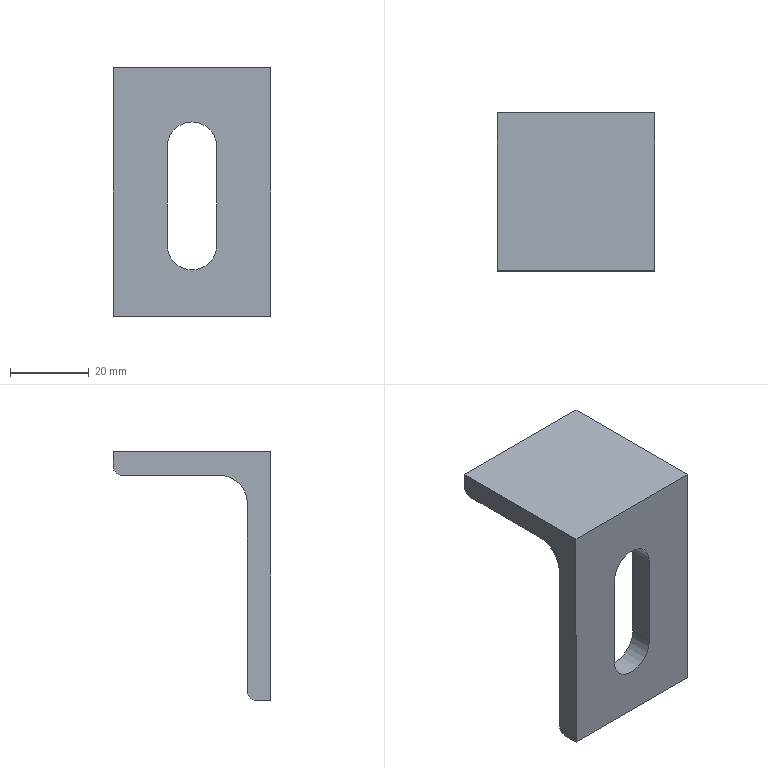Part | SolidWorks | features 3DProfileFeature 1, Cut 1, WeldMemberFeat 1, WeldmentFeature 1 | 1 solid | 16 faces | box 40 x 40 x 63 mm | volume 20996 mm3 | plane 10 | cylinder 6 | commonest cylinder face diameters 12.5 x3 4.667 x2 14 x1
STEP:
#1=CARTESIAN_POINT('',(200.,114.,-13.75));
#2=VERTEX_POINT('',#1);
#3=CARTESIAN_POINT('',(206.25,114.,-20.));
#4=VERTEX_POINT('',#3);
#5=CARTESIAN_POINT('',(200.,114.,-20.));
#6=DIRECTION('',(0.,1.,0.));
#7=DIRECTION('',(0.,0.,1.));
#8=AXIS2_PLACEMENT_3D('',#5,#6,#7);
#9=CIRCLE('',#8,6.25);
#10=EDGE_CURVE('',#2,#4,#9,.T.);
#11=ORIENTED_EDGE('',*,*,#10,.F.);
#12=CARTESIAN_POINT('',(200.,120.,-13.75));
#13=VERTEX_POINT('',#12);
#14=CARTESIAN_POINT('',(200.,110.,-13.75));
#15=DIRECTION('',(0.,1.,0.));
#16=VECTOR('',#15,1000.);
#17=LINE('',#14,#16);
#18=EDGE_CURVE('',#2,#13,#17,.T.);
#19=ORIENTED_EDGE('',*,*,#18,.T.);
#20=CARTESIAN_POINT('',(206.25,120.,-20.));
#21=VERTEX_POINT('',#20);
#22=CARTESIAN_POINT('',(200.,120.,-20.));
#23=DIRECTION('',(0.,1.,0.));
#24=DIRECTION('',(0.,0.,1.));
#25=AXIS2_PLACEMENT_3D('',#22,#23,#24);
#26=CIRCLE('',#25,6.25);
#27=EDGE_CURVE('',#13,#21,#26,.T.);
#28=ORIENTED_EDGE('',*,*,#27,.T.);
#29=CARTESIAN_POINT('',(206.25,110.,-20.));
#30=DIRECTION('',(0.,1.,0.));
#31=VECTOR('',#30,1000.);
#32=LINE('',#29,#31);
#33=EDGE_CURVE('',#4,#21,#32,.T.);
#34=ORIENTED_EDGE('',*,*,#33,.F.);
#35=EDGE_LOOP('',(#11,#19,#28,#34));
#36=FACE_OUTER_BOUND('',#35,.T.);
#37=CARTESIAN_POINT('',(200.,110.,-20.));
#38=DIRECTION('',(0.,1.,0.));
#39=DIRECTION('',(0.,0.,1.));
#40=AXIS2_PLACEMENT_3D('',#37,#38,#39);
#41=CYLINDRICAL_SURFACE('',#40,6.25);
#42=ADVANCED_FACE('',(#36),#41,.F.);
#43=CARTESIAN_POINT('',(220.,114.,0.));
#44=VERTEX_POINT('',#43);
#45=CARTESIAN_POINT('',(220.,154.,0.));
#46=VERTEX_POINT('',#45);
#47=CARTESIAN_POINT('',(220.,154.,0.));
#48=DIRECTION('',(0.,1.,0.));
#49=VECTOR('',#48,1000.);
#50=LINE('',#47,#49);
#51=EDGE_CURVE('',#44,#46,#50,.T.);
#52=ORIENTED_EDGE('',*,*,#51,.T.);
#53=CARTESIAN_POINT('',(180.,154.,0.));
#54=VERTEX_POINT('',#53);
#55=CARTESIAN_POINT('',(180.,154.,0.));
#56=DIRECTION('',(1.,0.,0.));
#57=VECTOR('',#56,1000.);
#58=LINE('',#55,#57);
#59=EDGE_CURVE('',#54,#46,#58,.T.);
#60=ORIENTED_EDGE('',*,*,#59,.F.);
#61=CARTESIAN_POINT('',(180.,114.,0.));
#62=VERTEX_POINT('',#61);
#63=CARTESIAN_POINT('',(180.,154.,0.));
#64=DIRECTION('',(0.,1.,0.));
#65=VECTOR('',#64,1000.);
#66=LINE('',#63,#65);
#67=EDGE_CURVE('',#62,#54,#66,.T.);
#68=ORIENTED_EDGE('',*,*,#67,.F.);
#69=CARTESIAN_POINT('',(180.,114.,0.));
#70=DIRECTION('',(1.,0.,0.));
#71=VECTOR('',#70,1000.);
#72=LINE('',#69,#71);
#73=EDGE_CURVE('',#62,#44,#72,.T.);
#74=ORIENTED_EDGE('',*,*,#73,.T.);
#75=EDGE_LOOP('',(#52,#60,#68,#74));
#76=FACE_OUTER_BOUND('',#75,.T.);
#77=CARTESIAN_POINT('',(180.,154.,0.));
#78=DIRECTION('',(0.,0.,-1.));
#79=DIRECTION('',(0.,1.,0.));
#80=AXIS2_PLACEMENT_3D('',#77,#78,#79);
#81=PLANE('',#80);
#82=ADVANCED_FACE('',(#76),#81,.F.);
#83=CARTESIAN_POINT('',(220.,154.,-3.667));
#84=VERTEX_POINT('',#83);
#85=CARTESIAN_POINT('',(220.,154.,0.));
#86=DIRECTION('',(0.,0.,-1.));
#87=VECTOR('',#86,1000.);
#88=LINE('',#85,#87);
#89=EDGE_CURVE('',#46,#84,#88,.T.);
#90=ORIENTED_EDGE('',*,*,#89,.T.);
#91=CARTESIAN_POINT('',(180.,154.,-3.667));
#92=VERTEX_POINT('',#91);
#93=CARTESIAN_POINT('',(180.,154.,-3.667));
#94=DIRECTION('',(1.,0.,0.));
#95=VECTOR('',#94,1000.);
#96=LINE('',#93,#95);
#97=EDGE_CURVE('',#92,#84,#96,.T.);
#98=ORIENTED_EDGE('',*,*,#97,.F.);
#99=CARTESIAN_POINT('',(180.,154.,0.));
#100=DIRECTION('',(0.,0.,-1.));
#101=VECTOR('',#100,1000.);
#102=LINE('',#99,#101);
#103=EDGE_CURVE('',#54,#92,#102,.T.);
#104=ORIENTED_EDGE('',*,*,#103,.F.);
#105=ORIENTED_EDGE('',*,*,#59,.T.);
#106=EDGE_LOOP('',(#90,#98,#104,#105));
#107=FACE_OUTER_BOUND('',#106,.T.);
#108=CARTESIAN_POINT('',(180.,154.,0.));
#109=DIRECTION('',(0.,-1.,0.));
#110=DIRECTION('',(0.,0.,-1.));
#111=AXIS2_PLACEMENT_3D('',#108,#109,#110);
#112=PLANE('',#111);
#113=ADVANCED_FACE('',(#107),#112,.F.);
#114=CARTESIAN_POINT('',(220.,151.667,-6.));
#115=VERTEX_POINT('',#114);
#116=CARTESIAN_POINT('',(220.,151.667,-3.667));
#117=DIRECTION('',(-1.,0.,0.));
#118=DIRECTION('',(0.,0.,1.));
#119=AXIS2_PLACEMENT_3D('',#116,#117,#118);
#120=CIRCLE('',#119,2.333);
#121=EDGE_CURVE('',#84,#115,#120,.T.);
#122=ORIENTED_EDGE('',*,*,#121,.T.);
#123=CARTESIAN_POINT('',(180.,151.667,-6.));
#124=VERTEX_POINT('',#123);
#125=CARTESIAN_POINT('',(180.,151.667,-6.));
#126=DIRECTION('',(1.,0.,0.));
#127=VECTOR('',#126,1000.);
#128=LINE('',#125,#127);
#129=EDGE_CURVE('',#124,#115,#128,.T.);
#130=ORIENTED_EDGE('',*,*,#129,.F.);
#131=CARTESIAN_POINT('',(180.,151.667,-3.667));
#132=DIRECTION('',(-1.,0.,0.));
#133=DIRECTION('',(0.,0.,1.));
#134=AXIS2_PLACEMENT_3D('',#131,#132,#133);
#135=CIRCLE('',#134,2.333);
#136=EDGE_CURVE('',#92,#124,#135,.T.);
#137=ORIENTED_EDGE('',*,*,#136,.F.);
#138=ORIENTED_EDGE('',*,*,#97,.T.);
#139=EDGE_LOOP('',(#122,#130,#137,#138));
#140=FACE_OUTER_BOUND('',#139,.T.);
#141=CARTESIAN_POINT('',(180.,151.667,-3.667));
#142=DIRECTION('',(1.,0.,0.));
#143=DIRECTION('',(0.,0.,-1.));
#144=AXIS2_PLACEMENT_3D('',#141,#142,#143);
#145=CYLINDRICAL_SURFACE('',#144,2.333);
#146=ADVANCED_FACE('',(#140),#145,.T.);
#147=CARTESIAN_POINT('',(220.,127.,-6.));
#148=VERTEX_POINT('',#147);
#149=CARTESIAN_POINT('',(220.,127.,-6.));
#150=DIRECTION('',(0.,-1.,0.));
#151=VECTOR('',#150,1000.);
#152=LINE('',#149,#151);
#153=EDGE_CURVE('',#115,#148,#152,.T.);
#154=ORIENTED_EDGE('',*,*,#153,.T.);
#155=CARTESIAN_POINT('',(180.,127.,-6.));
#156=VERTEX_POINT('',#155);
#157=CARTESIAN_POINT('',(180.,127.,-6.));
#158=DIRECTION('',(1.,0.,0.));
#159=VECTOR('',#158,1000.);
#160=LINE('',#157,#159);
#161=EDGE_CURVE('',#156,#148,#160,.T.);
#162=ORIENTED_EDGE('',*,*,#161,.F.);
#163=CARTESIAN_POINT('',(180.,127.,-6.));
#164=DIRECTION('',(0.,-1.,0.));
#165=VECTOR('',#164,1000.);
#166=LINE('',#163,#165);
#167=EDGE_CURVE('',#124,#156,#166,.T.);
#168=ORIENTED_EDGE('',*,*,#167,.F.);
#169=ORIENTED_EDGE('',*,*,#129,.T.);
#170=EDGE_LOOP('',(#154,#162,#168,#169));
#171=FACE_OUTER_BOUND('',#170,.T.);
#172=CARTESIAN_POINT('',(180.,127.,-6.));
#173=DIRECTION('',(0.,0.,1.));
#174=DIRECTION('',(0.,-1.,0.));
#175=AXIS2_PLACEMENT_3D('',#172,#173,#174);
#176=PLANE('',#175);
#177=ADVANCED_FACE('',(#171),#176,.F.);
#178=CARTESIAN_POINT('',(220.,120.,-13.));
#179=VERTEX_POINT('',#178);
#180=CARTESIAN_POINT('',(220.,127.,-13.));
#181=DIRECTION('',(1.,0.,0.));
#182=DIRECTION('',(0.,0.,-1.));
#183=AXIS2_PLACEMENT_3D('',#180,#181,#182);
#184=CIRCLE('',#183,7.);
#185=EDGE_CURVE('',#148,#179,#184,.T.);
#186=ORIENTED_EDGE('',*,*,#185,.T.);
#187=CARTESIAN_POINT('',(180.,120.,-13.));
#188=VERTEX_POINT('',#187);
#189=CARTESIAN_POINT('',(180.,120.,-13.));
#190=DIRECTION('',(1.,0.,0.));
#191=VECTOR('',#190,1000.);
#192=LINE('',#189,#191);
#193=EDGE_CURVE('',#188,#179,#192,.T.);
#194=ORIENTED_EDGE('',*,*,#193,.F.);
#195=CARTESIAN_POINT('',(180.,127.,-13.));
#196=DIRECTION('',(1.,0.,0.));
#197=DIRECTION('',(0.,0.,-1.));
#198=AXIS2_PLACEMENT_3D('',#195,#196,#197);
#199=CIRCLE('',#198,7.);
#200=EDGE_CURVE('',#156,#188,#199,.T.);
#201=ORIENTED_EDGE('',*,*,#200,.F.);
#202=ORIENTED_EDGE('',*,*,#161,.T.);
#203=EDGE_LOOP('',(#186,#194,#201,#202));
#204=FACE_OUTER_BOUND('',#203,.T.);
#205=CARTESIAN_POINT('',(180.,127.,-13.));
#206=DIRECTION('',(1.,0.,0.));
#207=DIRECTION('',(0.,0.,-1.));
#208=AXIS2_PLACEMENT_3D('',#205,#206,#207);
#209=CYLINDRICAL_SURFACE('',#208,7.);
#210=ADVANCED_FACE('',(#204),#209,.F.);
#211=CARTESIAN_POINT('',(193.75,120.,-45.));
#212=VERTEX_POINT('',#211);
#213=CARTESIAN_POINT('',(193.75,120.,-20.));
#214=VERTEX_POINT('',#213);
#215=CARTESIAN_POINT('',(193.75,120.,-45.));
#216=DIRECTION('',(0.,0.,1.));
#217=VECTOR('',#216,1000.);
#218=LINE('',#215,#217);
#219=EDGE_CURVE('',#212,#214,#218,.T.);
#220=ORIENTED_EDGE('',*,*,#219,.F.);
#221=CARTESIAN_POINT('',(206.25,120.,-45.));
#222=VERTEX_POINT('',#221);
#223=CARTESIAN_POINT('',(200.,120.,-45.));
#224=DIRECTION('',(0.,1.,0.));
#225=DIRECTION('',(0.,0.,1.));
#226=AXIS2_PLACEMENT_3D('',#223,#224,#225);
#227=CIRCLE('',#226,6.25);
#228=EDGE_CURVE('',#222,#212,#227,.T.);
#229=ORIENTED_EDGE('',*,*,#228,.F.);
#230=CARTESIAN_POINT('',(206.25,120.,-45.));
#231=DIRECTION('',(0.,0.,-1.));
#232=VECTOR('',#231,1000.);
#233=LINE('',#230,#232);
#234=EDGE_CURVE('',#21,#222,#233,.T.);
#235=ORIENTED_EDGE('',*,*,#234,.F.);
#236=ORIENTED_EDGE('',*,*,#27,.F.);
#237=CARTESIAN_POINT('',(200.,120.,-20.));
#238=DIRECTION('',(0.,1.,0.));
#239=DIRECTION('',(0.,0.,1.));
#240=AXIS2_PLACEMENT_3D('',#237,#238,#239);
#241=CIRCLE('',#240,6.25);
#242=EDGE_CURVE('',#214,#13,#241,.T.);
#243=ORIENTED_EDGE('',*,*,#242,.F.);
#244=EDGE_LOOP('',(#220,#229,#235,#236,#243));
#245=FACE_BOUND('',#244,.T.);
#246=CARTESIAN_POINT('',(220.,120.,-60.667));
#247=VERTEX_POINT('',#246);
#248=CARTESIAN_POINT('',(220.,120.,-60.667));
#249=DIRECTION('',(0.,0.,-1.));
#250=VECTOR('',#249,1000.);
#251=LINE('',#248,#250);
#252=EDGE_CURVE('',#179,#247,#251,.T.);
#253=ORIENTED_EDGE('',*,*,#252,.T.);
#254=CARTESIAN_POINT('',(180.,120.,-60.667));
#255=VERTEX_POINT('',#254);
#256=CARTESIAN_POINT('',(180.,120.,-60.667));
#257=DIRECTION('',(1.,0.,0.));
#258=VECTOR('',#257,1000.);
#259=LINE('',#256,#258);
#260=EDGE_CURVE('',#255,#247,#259,.T.);
#261=ORIENTED_EDGE('',*,*,#260,.F.);
#262=CARTESIAN_POINT('',(180.,120.,-60.667));
#263=DIRECTION('',(0.,0.,-1.));
#264=VECTOR('',#263,1000.);
#265=LINE('',#262,#264);
#266=EDGE_CURVE('',#188,#255,#265,.T.);
#267=ORIENTED_EDGE('',*,*,#266,.F.);
#268=ORIENTED_EDGE('',*,*,#193,.T.);
#269=EDGE_LOOP('',(#253,#261,#267,#268));
#270=FACE_OUTER_BOUND('',#269,.T.);
#271=CARTESIAN_POINT('',(180.,120.,-60.667));
#272=DIRECTION('',(0.,-1.,0.));
#273=DIRECTION('',(0.,0.,-1.));
#274=AXIS2_PLACEMENT_3D('',#271,#272,#273);
#275=PLANE('',#274);
#276=ADVANCED_FACE('',(#245,#270),#275,.F.);
#277=CARTESIAN_POINT('',(220.,117.667,-63.));
#278=VERTEX_POINT('',#277);
#279=CARTESIAN_POINT('',(220.,117.667,-60.667));
#280=DIRECTION('',(-1.,0.,0.));
#281=DIRECTION('',(0.,0.,-1.));
#282=AXIS2_PLACEMENT_3D('',#279,#280,#281);
#283=CIRCLE('',#282,2.333);
#284=EDGE_CURVE('',#247,#278,#283,.T.);
#285=ORIENTED_EDGE('',*,*,#284,.T.);
#286=CARTESIAN_POINT('',(180.,117.667,-63.));
#287=VERTEX_POINT('',#286);
#288=CARTESIAN_POINT('',(180.,117.667,-63.));
#289=DIRECTION('',(1.,0.,0.));
#290=VECTOR('',#289,1000.);
#291=LINE('',#288,#290);
#292=EDGE_CURVE('',#287,#278,#291,.T.);
#293=ORIENTED_EDGE('',*,*,#292,.F.);
#294=CARTESIAN_POINT('',(180.,117.667,-60.667));
#295=DIRECTION('',(-1.,0.,0.));
#296=DIRECTION('',(0.,0.,-1.));
#297=AXIS2_PLACEMENT_3D('',#294,#295,#296);
#298=CIRCLE('',#297,2.333);
#299=EDGE_CURVE('',#255,#287,#298,.T.);
#300=ORIENTED_EDGE('',*,*,#299,.F.);
#301=ORIENTED_EDGE('',*,*,#260,.T.);
#302=EDGE_LOOP('',(#285,#293,#300,#301));
#303=FACE_OUTER_BOUND('',#302,.T.);
#304=CARTESIAN_POINT('',(180.,117.667,-60.667));
#305=DIRECTION('',(1.,0.,0.));
#306=DIRECTION('',(0.,0.,-1.));
#307=AXIS2_PLACEMENT_3D('',#304,#305,#306);
#308=CYLINDRICAL_SURFACE('',#307,2.333);
#309=ADVANCED_FACE('',(#303),#308,.T.);
#310=CARTESIAN_POINT('',(220.,114.,-63.));
#311=VERTEX_POINT('',#310);
#312=CARTESIAN_POINT('',(220.,114.,-63.));
#313=DIRECTION('',(0.,-1.,0.));
#314=VECTOR('',#313,1000.);
#315=LINE('',#312,#314);
#316=EDGE_CURVE('',#278,#311,#315,.T.);
#317=ORIENTED_EDGE('',*,*,#316,.T.);
#318=CARTESIAN_POINT('',(180.,114.,-63.));
#319=VERTEX_POINT('',#318);
#320=CARTESIAN_POINT('',(180.,114.,-63.));
#321=DIRECTION('',(1.,0.,0.));
#322=VECTOR('',#321,1000.);
#323=LINE('',#320,#322);
#324=EDGE_CURVE('',#319,#311,#323,.T.);
#325=ORIENTED_EDGE('',*,*,#324,.F.);
#326=CARTESIAN_POINT('',(180.,114.,-63.));
#327=DIRECTION('',(0.,-1.,0.));
#328=VECTOR('',#327,1000.);
#329=LINE('',#326,#328);
#330=EDGE_CURVE('',#287,#319,#329,.T.);
#331=ORIENTED_EDGE('',*,*,#330,.F.);
#332=ORIENTED_EDGE('',*,*,#292,.T.);
#333=EDGE_LOOP('',(#317,#325,#331,#332));
#334=FACE_OUTER_BOUND('',#333,.T.);
#335=CARTESIAN_POINT('',(180.,114.,-63.));
#336=DIRECTION('',(0.,0.,1.));
#337=DIRECTION('',(0.,-1.,0.));
#338=AXIS2_PLACEMENT_3D('',#335,#336,#337);
#339=PLANE('',#338);
#340=ADVANCED_FACE('',(#334),#339,.F.);
#341=CARTESIAN_POINT('',(206.25,114.,-45.));
#342=VERTEX_POINT('',#341);
#343=CARTESIAN_POINT('',(206.25,114.,0.));
#344=DIRECTION('',(0.,0.,-1.));
#345=VECTOR('',#344,1000.);
#346=LINE('',#343,#345);
#347=EDGE_CURVE('',#4,#342,#346,.T.);
#348=ORIENTED_EDGE('',*,*,#347,.T.);
#349=CARTESIAN_POINT('',(193.75,114.,-45.));
#350=VERTEX_POINT('',#349);
#351=CARTESIAN_POINT('',(200.,114.,-45.));
#352=DIRECTION('',(0.,1.,0.));
#353=DIRECTION('',(0.,0.,1.));
#354=AXIS2_PLACEMENT_3D('',#351,#352,#353);
#355=CIRCLE('',#354,6.25);
#356=EDGE_CURVE('',#342,#350,#355,.T.);
#357=ORIENTED_EDGE('',*,*,#356,.T.);
#358=CARTESIAN_POINT('',(193.75,114.,-20.));
#359=VERTEX_POINT('',#358);
#360=CARTESIAN_POINT('',(193.75,114.,0.));
#361=DIRECTION('',(0.,0.,1.));
#362=VECTOR('',#361,1000.);
#363=LINE('',#360,#362);
#364=EDGE_CURVE('',#350,#359,#363,.T.);
#365=ORIENTED_EDGE('',*,*,#364,.T.);
#366=CARTESIAN_POINT('',(200.,114.,-20.));
#367=DIRECTION('',(0.,1.,0.));
#368=DIRECTION('',(0.,0.,1.));
#369=AXIS2_PLACEMENT_3D('',#366,#367,#368);
#370=CIRCLE('',#369,6.25);
#371=EDGE_CURVE('',#359,#2,#370,.T.);
#372=ORIENTED_EDGE('',*,*,#371,.T.);
#373=ORIENTED_EDGE('',*,*,#10,.T.);
#374=EDGE_LOOP('',(#348,#357,#365,#372,#373));
#375=FACE_BOUND('',#374,.T.);
#376=CARTESIAN_POINT('',(220.,114.,0.));
#377=DIRECTION('',(0.,0.,1.));
#378=VECTOR('',#377,1000.);
#379=LINE('',#376,#378);
#380=EDGE_CURVE('',#311,#44,#379,.T.);
#381=ORIENTED_EDGE('',*,*,#380,.T.);
#382=ORIENTED_EDGE('',*,*,#73,.F.);
#383=CARTESIAN_POINT('',(180.,114.,0.));
#384=DIRECTION('',(0.,0.,1.));
#385=VECTOR('',#384,1000.);
#386=LINE('',#383,#385);
#387=EDGE_CURVE('',#319,#62,#386,.T.);
#388=ORIENTED_EDGE('',*,*,#387,.F.);
#389=ORIENTED_EDGE('',*,*,#324,.T.);
#390=EDGE_LOOP('',(#381,#382,#388,#389));
#391=FACE_OUTER_BOUND('',#390,.T.);
#392=CARTESIAN_POINT('',(180.,114.,0.));
#393=DIRECTION('',(0.,1.,0.));
#394=DIRECTION('',(0.,0.,1.));
#395=AXIS2_PLACEMENT_3D('',#392,#393,#394);
#396=PLANE('',#395);
#397=ADVANCED_FACE('',(#375,#391),#396,.F.);
#398=ORIENTED_EDGE('',*,*,#67,.T.);
#399=ORIENTED_EDGE('',*,*,#103,.T.);
#400=ORIENTED_EDGE('',*,*,#136,.T.);
#401=ORIENTED_EDGE('',*,*,#167,.T.);
#402=ORIENTED_EDGE('',*,*,#200,.T.);
#403=ORIENTED_EDGE('',*,*,#266,.T.);
#404=ORIENTED_EDGE('',*,*,#299,.T.);
#405=ORIENTED_EDGE('',*,*,#330,.T.);
#406=ORIENTED_EDGE('',*,*,#387,.T.);
#407=EDGE_LOOP('',(#398,#399,#400,#401,#402,#403,#404,#405,#406));
#408=FACE_OUTER_BOUND('',#407,.T.);
#409=CARTESIAN_POINT('',(180.,117.667,-60.667));
#410=DIRECTION('',(1.,0.,0.));
#411=DIRECTION('',(0.,0.,-1.));
#412=AXIS2_PLACEMENT_3D('',#409,#410,#411);
#413=PLANE('',#412);
#414=ADVANCED_FACE('',(#408),#413,.F.);
#415=ORIENTED_EDGE('',*,*,#51,.F.);
#416=ORIENTED_EDGE('',*,*,#380,.F.);
#417=ORIENTED_EDGE('',*,*,#316,.F.);
#418=ORIENTED_EDGE('',*,*,#284,.F.);
#419=ORIENTED_EDGE('',*,*,#252,.F.);
#420=ORIENTED_EDGE('',*,*,#185,.F.);
#421=ORIENTED_EDGE('',*,*,#153,.F.);
#422=ORIENTED_EDGE('',*,*,#121,.F.);
#423=ORIENTED_EDGE('',*,*,#89,.F.);
#424=EDGE_LOOP('',(#415,#416,#417,#418,#419,#420,#421,#422,#423));
#425=FACE_OUTER_BOUND('',#424,.T.);
#426=CARTESIAN_POINT('',(220.,117.667,-60.667));
#427=DIRECTION('',(1.,0.,0.));
#428=DIRECTION('',(0.,0.,-1.));
#429=AXIS2_PLACEMENT_3D('',#426,#427,#428);
#430=PLANE('',#429);
#431=ADVANCED_FACE('',(#425),#430,.T.);
#432=CARTESIAN_POINT('',(206.25,110.,-45.));
#433=DIRECTION('',(0.,1.,0.));
#434=VECTOR('',#433,1000.);
#435=LINE('',#432,#434);
#436=EDGE_CURVE('',#342,#222,#435,.T.);
#437=ORIENTED_EDGE('',*,*,#436,.T.);
#438=ORIENTED_EDGE('',*,*,#228,.T.);
#439=CARTESIAN_POINT('',(193.75,110.,-45.));
#440=DIRECTION('',(0.,1.,0.));
#441=VECTOR('',#440,1000.);
#442=LINE('',#439,#441);
#443=EDGE_CURVE('',#350,#212,#442,.T.);
#444=ORIENTED_EDGE('',*,*,#443,.F.);
#445=ORIENTED_EDGE('',*,*,#356,.F.);
#446=EDGE_LOOP('',(#437,#438,#444,#445));
#447=FACE_OUTER_BOUND('',#446,.T.);
#448=CARTESIAN_POINT('',(200.,110.,-45.));
#449=DIRECTION('',(0.,1.,0.));
#450=DIRECTION('',(0.,0.,1.));
#451=AXIS2_PLACEMENT_3D('',#448,#449,#450);
#452=CYLINDRICAL_SURFACE('',#451,6.25);
#453=ADVANCED_FACE('',(#447),#452,.F.);
#454=ORIENTED_EDGE('',*,*,#33,.T.);
#455=ORIENTED_EDGE('',*,*,#234,.T.);
#456=ORIENTED_EDGE('',*,*,#436,.F.);
#457=ORIENTED_EDGE('',*,*,#347,.F.);
#458=EDGE_LOOP('',(#454,#455,#456,#457));
#459=FACE_OUTER_BOUND('',#458,.T.);
#460=CARTESIAN_POINT('',(206.25,110.,-45.));
#461=DIRECTION('',(1.,0.,0.));
#462=DIRECTION('',(0.,0.,-1.));
#463=AXIS2_PLACEMENT_3D('',#460,#461,#462);
#464=PLANE('',#463);
#465=ADVANCED_FACE('',(#459),#464,.F.);
#466=ORIENTED_EDGE('',*,*,#18,.F.);
#467=ORIENTED_EDGE('',*,*,#371,.F.);
#468=CARTESIAN_POINT('',(193.75,110.,-20.));
#469=DIRECTION('',(0.,1.,0.));
#470=VECTOR('',#469,1000.);
#471=LINE('',#468,#470);
#472=EDGE_CURVE('',#359,#214,#471,.T.);
#473=ORIENTED_EDGE('',*,*,#472,.T.);
#474=ORIENTED_EDGE('',*,*,#242,.T.);
#475=EDGE_LOOP('',(#466,#467,#473,#474));
#476=FACE_OUTER_BOUND('',#475,.T.);
#477=CARTESIAN_POINT('',(200.,110.,-20.));
#478=DIRECTION('',(0.,1.,0.));
#479=DIRECTION('',(0.,0.,1.));
#480=AXIS2_PLACEMENT_3D('',#477,#478,#479);
#481=CYLINDRICAL_SURFACE('',#480,6.25);
#482=ADVANCED_FACE('',(#476),#481,.F.);
#483=ORIENTED_EDGE('',*,*,#443,.T.);
#484=ORIENTED_EDGE('',*,*,#219,.T.);
#485=ORIENTED_EDGE('',*,*,#472,.F.);
#486=ORIENTED_EDGE('',*,*,#364,.F.);
#487=EDGE_LOOP('',(#483,#484,#485,#486));
#488=FACE_OUTER_BOUND('',#487,.T.);
#489=CARTESIAN_POINT('',(193.75,110.,-45.));
#490=DIRECTION('',(-1.,0.,0.));
#491=DIRECTION('',(0.,0.,1.));
#492=AXIS2_PLACEMENT_3D('',#489,#490,#491);
#493=PLANE('',#492);
#494=ADVANCED_FACE('',(#488),#493,.F.);
#495=CLOSED_SHELL('',(#42,#82,#113,#146,#177,#210,#276,#309,#340,#397,#414,#431,#453,#465,#482,#494));
#496=MANIFOLD_SOLID_BREP('',#495);
#497=CARTESIAN_POINT('',(0.,0.,0.));
#498=DIRECTION('',(0.,0.,1.));
#499=DIRECTION('',(1.,0.,0.));
#500=AXIS2_PLACEMENT_3D('',#497,#498,#499);
#501=(LENGTH_UNIT()NAMED_UNIT(*)SI_UNIT(.MILLI.,.METRE.));
#502=UNCERTAINTY_MEASURE_WITH_UNIT(LENGTH_MEASURE(0.00001),#501,'','');
#503=(NAMED_UNIT(*)PLANE_ANGLE_UNIT()SI_UNIT($,.RADIAN.));
#504=(NAMED_UNIT(*)SI_UNIT($,.STERADIAN.)SOLID_ANGLE_UNIT());
#505=(GEOMETRIC_REPRESENTATION_CONTEXT(3)GLOBAL_UNCERTAINTY_ASSIGNED_CONTEXT((#502))GLOBAL_UNIT_ASSIGNED_CONTEXT((#501,#503,#504))REPRESENTATION_CONTEXT('',''));
#506=ADVANCED_BREP_SHAPE_REPRESENTATION('',(#496,#500),#505);